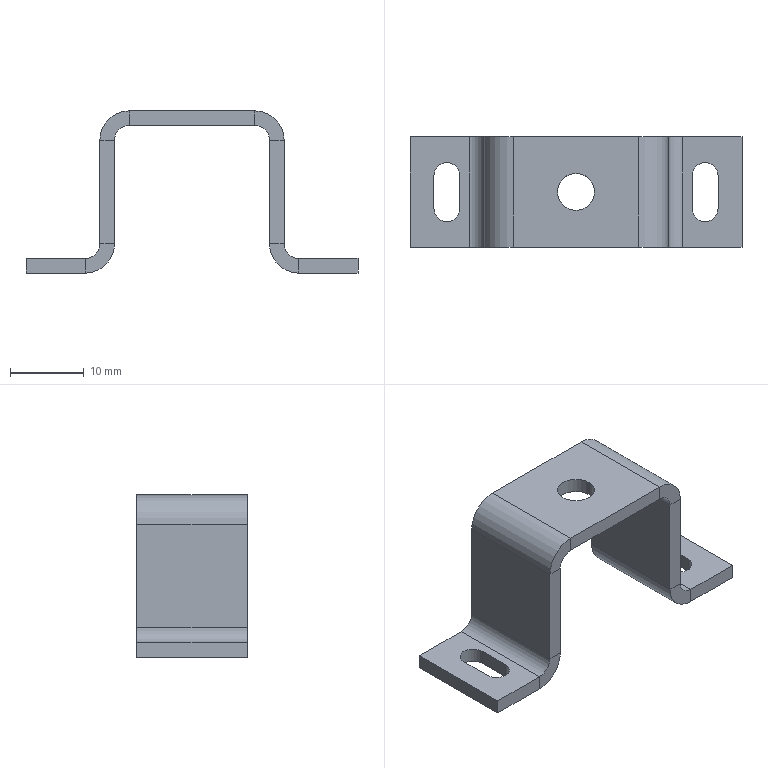Part | STEP file | Lead screw connecting block V1.201001 | 1 solid | 48 faces | box 45 x 15 x 22 mm | volume 2255 mm3 | plane 34 | cylinder 14 | commonest cylinder face diameters 3.5 x4 4 x4 8 x4 5 x2